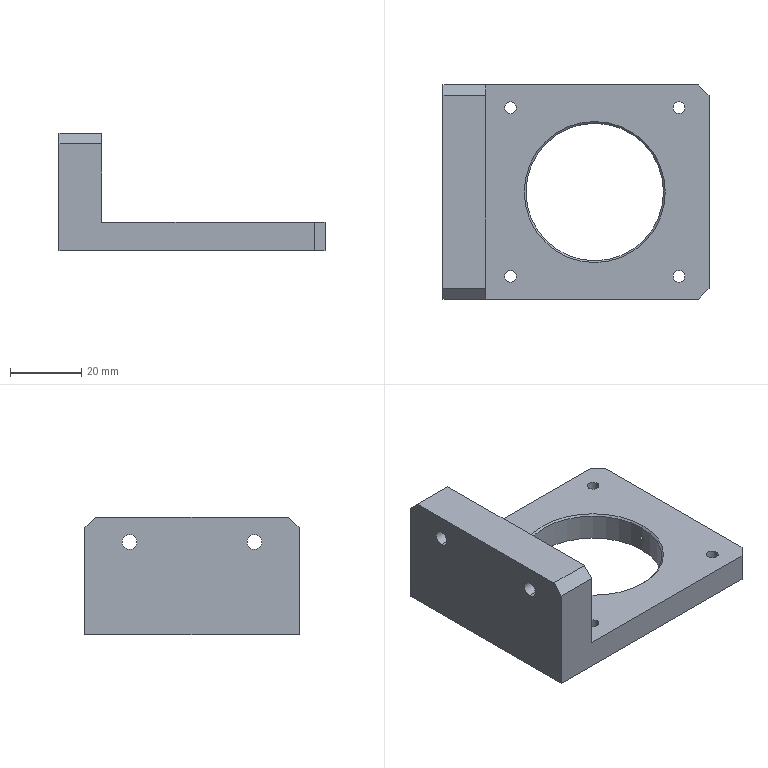Part | NX | features BREP 1 | 1 solid | 32 faces | box 74.5 x 60 x 33 mm | volume 43539 mm3 | cylinder 16 | plane 12 | cone 4 | commonest cylinder face diameters 3.3 x10 4.2 x4 38.5 x2
STEP:
#1=CARTESIAN_POINT('',(-42.5,-30.,30.));
#2=VERTEX_POINT('',#1);
#3=CARTESIAN_POINT('',(-42.5,-27.,33.));
#4=VERTEX_POINT('',#3);
#5=CARTESIAN_POINT('',(-42.5,-27.,33.));
#6=DIRECTION('',(0.,0.7071,0.7071));
#7=VECTOR('',#6,1000.);
#8=LINE('',#5,#7);
#9=EDGE_CURVE('',#2,#4,#8,.T.);
#10=ORIENTED_EDGE('',*,*,#9,.F.);
#11=CARTESIAN_POINT('',(-30.5,-30.,30.));
#12=VERTEX_POINT('',#11);
#13=CARTESIAN_POINT('',(-42.5,-30.,30.));
#14=DIRECTION('',(-1.,0.,0.));
#15=VECTOR('',#14,1000.);
#16=LINE('',#13,#15);
#17=EDGE_CURVE('',#12,#2,#16,.T.);
#18=ORIENTED_EDGE('',*,*,#17,.F.);
#19=CARTESIAN_POINT('',(-30.5,-27.,33.));
#20=VERTEX_POINT('',#19);
#21=CARTESIAN_POINT('',(-30.5,-27.,33.));
#22=DIRECTION('',(0.,-0.7071,-0.7071));
#23=VECTOR('',#22,1000.);
#24=LINE('',#21,#23);
#25=EDGE_CURVE('',#20,#12,#24,.T.);
#26=ORIENTED_EDGE('',*,*,#25,.F.);
#27=CARTESIAN_POINT('',(-30.5,-27.,33.));
#28=DIRECTION('',(1.,0.,0.));
#29=VECTOR('',#28,1000.);
#30=LINE('',#27,#29);
#31=EDGE_CURVE('',#4,#20,#30,.T.);
#32=ORIENTED_EDGE('',*,*,#31,.F.);
#33=EDGE_LOOP('',(#10,#18,#26,#32));
#34=FACE_BOUND('',#33,.T.);
#35=CARTESIAN_POINT('',(0.,-27.,33.));
#36=DIRECTION('',(0.,-0.7071,0.7071));
#37=DIRECTION('',(-1.,0.,0.));
#38=AXIS2_PLACEMENT_3D('',#35,#36,#37);
#39=PLANE('',#38);
#40=ADVANCED_FACE('',(#34),#39,.T.);
#41=CARTESIAN_POINT('',(-30.5,30.,30.));
#42=VERTEX_POINT('',#41);
#43=CARTESIAN_POINT('',(-30.5,27.,33.));
#44=VERTEX_POINT('',#43);
#45=CARTESIAN_POINT('',(-30.5,27.,33.));
#46=DIRECTION('',(0.,-0.7071,0.7071));
#47=VECTOR('',#46,1000.);
#48=LINE('',#45,#47);
#49=EDGE_CURVE('',#42,#44,#48,.T.);
#50=ORIENTED_EDGE('',*,*,#49,.F.);
#51=CARTESIAN_POINT('',(-42.5,30.,30.));
#52=VERTEX_POINT('',#51);
#53=CARTESIAN_POINT('',(-30.5,30.,30.));
#54=DIRECTION('',(1.,0.,0.));
#55=VECTOR('',#54,1000.);
#56=LINE('',#53,#55);
#57=EDGE_CURVE('',#52,#42,#56,.T.);
#58=ORIENTED_EDGE('',*,*,#57,.F.);
#59=CARTESIAN_POINT('',(-42.5,27.,33.));
#60=VERTEX_POINT('',#59);
#61=CARTESIAN_POINT('',(-42.5,27.,33.));
#62=DIRECTION('',(0.,0.7071,-0.7071));
#63=VECTOR('',#62,1000.);
#64=LINE('',#61,#63);
#65=EDGE_CURVE('',#60,#52,#64,.T.);
#66=ORIENTED_EDGE('',*,*,#65,.F.);
#67=CARTESIAN_POINT('',(-42.5,27.,33.));
#68=DIRECTION('',(-1.,0.,0.));
#69=VECTOR('',#68,1000.);
#70=LINE('',#67,#69);
#71=EDGE_CURVE('',#44,#60,#70,.T.);
#72=ORIENTED_EDGE('',*,*,#71,.F.);
#73=EDGE_LOOP('',(#50,#58,#66,#72));
#74=FACE_BOUND('',#73,.T.);
#75=CARTESIAN_POINT('',(0.,27.,33.));
#76=DIRECTION('',(0.,0.7071,0.7071));
#77=DIRECTION('',(1.,0.,0.));
#78=AXIS2_PLACEMENT_3D('',#75,#76,#77);
#79=PLANE('',#78);
#80=ADVANCED_FACE('',(#74),#79,.T.);
#81=CARTESIAN_POINT('',(29.,-30.,8.));
#82=VERTEX_POINT('',#81);
#83=CARTESIAN_POINT('',(32.,-27.,8.));
#84=VERTEX_POINT('',#83);
#85=CARTESIAN_POINT('',(32.,-27.,8.));
#86=DIRECTION('',(0.7071,0.7071,0.));
#87=VECTOR('',#86,1000.);
#88=LINE('',#85,#87);
#89=EDGE_CURVE('',#82,#84,#88,.T.);
#90=ORIENTED_EDGE('',*,*,#89,.F.);
#91=CARTESIAN_POINT('',(29.,-30.,0.));
#92=VERTEX_POINT('',#91);
#93=CARTESIAN_POINT('',(29.,-30.,8.));
#94=DIRECTION('',(0.,0.,1.));
#95=VECTOR('',#94,1000.);
#96=LINE('',#93,#95);
#97=EDGE_CURVE('',#92,#82,#96,.T.);
#98=ORIENTED_EDGE('',*,*,#97,.F.);
#99=CARTESIAN_POINT('',(32.,-27.,0.));
#100=VERTEX_POINT('',#99);
#101=CARTESIAN_POINT('',(29.5,-29.5,0.));
#102=DIRECTION('',(-0.7071,-0.7071,0.));
#103=VECTOR('',#102,1000.);
#104=LINE('',#101,#103);
#105=EDGE_CURVE('',#100,#92,#104,.T.);
#106=ORIENTED_EDGE('',*,*,#105,.F.);
#107=CARTESIAN_POINT('',(32.,-27.,8.));
#108=DIRECTION('',(0.,0.,-1.));
#109=VECTOR('',#108,1000.);
#110=LINE('',#107,#109);
#111=EDGE_CURVE('',#84,#100,#110,.T.);
#112=ORIENTED_EDGE('',*,*,#111,.F.);
#113=EDGE_LOOP('',(#90,#98,#106,#112));
#114=FACE_BOUND('',#113,.T.);
#115=CARTESIAN_POINT('',(32.,-27.,8.));
#116=DIRECTION('',(-0.7071,0.7071,0.));
#117=DIRECTION('',(0.,0.,-1.));
#118=AXIS2_PLACEMENT_3D('',#115,#116,#117);
#119=PLANE('',#118);
#120=ADVANCED_FACE('',(#114),#119,.F.);
#121=CARTESIAN_POINT('',(32.,27.,8.));
#122=VERTEX_POINT('',#121);
#123=CARTESIAN_POINT('',(29.,30.,8.));
#124=VERTEX_POINT('',#123);
#125=CARTESIAN_POINT('',(29.,30.,8.));
#126=DIRECTION('',(-0.7071,0.7071,0.));
#127=VECTOR('',#126,1000.);
#128=LINE('',#125,#127);
#129=EDGE_CURVE('',#122,#124,#128,.T.);
#130=ORIENTED_EDGE('',*,*,#129,.F.);
#131=CARTESIAN_POINT('',(32.,27.,0.));
#132=VERTEX_POINT('',#131);
#133=CARTESIAN_POINT('',(32.,27.,8.));
#134=DIRECTION('',(0.,0.,1.));
#135=VECTOR('',#134,1000.);
#136=LINE('',#133,#135);
#137=EDGE_CURVE('',#132,#122,#136,.T.);
#138=ORIENTED_EDGE('',*,*,#137,.F.);
#139=CARTESIAN_POINT('',(29.,30.,0.));
#140=VERTEX_POINT('',#139);
#141=CARTESIAN_POINT('',(29.5,29.5,0.));
#142=DIRECTION('',(0.7071,-0.7071,0.));
#143=VECTOR('',#142,1000.);
#144=LINE('',#141,#143);
#145=EDGE_CURVE('',#140,#132,#144,.T.);
#146=ORIENTED_EDGE('',*,*,#145,.F.);
#147=CARTESIAN_POINT('',(29.,30.,8.));
#148=DIRECTION('',(0.,0.,-1.));
#149=VECTOR('',#148,1000.);
#150=LINE('',#147,#149);
#151=EDGE_CURVE('',#124,#140,#150,.T.);
#152=ORIENTED_EDGE('',*,*,#151,.F.);
#153=EDGE_LOOP('',(#130,#138,#146,#152));
#154=FACE_BOUND('',#153,.T.);
#155=CARTESIAN_POINT('',(29.,30.,8.));
#156=DIRECTION('',(-0.7071,-0.7071,0.));
#157=DIRECTION('',(0.,0.,-1.));
#158=AXIS2_PLACEMENT_3D('',#155,#156,#157);
#159=PLANE('',#158);
#160=ADVANCED_FACE('',(#154),#159,.F.);
#161=CARTESIAN_POINT('',(19.9,0.,5.65));
#162=VERTEX_POINT('',#161);
#163=CARTESIAN_POINT('',(32.,0.,5.65));
#164=VERTEX_POINT('',#163);
#165=CARTESIAN_POINT('',(32.,0.,5.65));
#166=DIRECTION('',(1.,0.,0.));
#167=VECTOR('',#166,1000.);
#168=LINE('',#165,#167);
#169=EDGE_CURVE('',#162,#164,#168,.T.);
#170=ORIENTED_EDGE('',*,*,#169,.F.);
#171=CARTESIAN_POINT('',(19.9,0.,2.35));
#172=VERTEX_POINT('',#171);
#173=CARTESIAN_POINT('',(19.9,0.,4.));
#174=DIRECTION('',(1.,0.,0.));
#175=DIRECTION('',(0.,0.,-1.));
#176=AXIS2_PLACEMENT_3D('',#173,#174,#175);
#177=CIRCLE('',#176,1.65);
#178=EDGE_CURVE('',#172,#162,#177,.T.);
#179=ORIENTED_EDGE('',*,*,#178,.F.);
#180=CARTESIAN_POINT('',(32.,0.,2.35));
#181=VERTEX_POINT('',#180);
#182=CARTESIAN_POINT('',(32.,0.,2.35));
#183=DIRECTION('',(1.,0.,0.));
#184=VECTOR('',#183,1000.);
#185=LINE('',#182,#184);
#186=EDGE_CURVE('',#172,#181,#185,.T.);
#187=ORIENTED_EDGE('',*,*,#186,.T.);
#188=CARTESIAN_POINT('',(32.,0.,4.));
#189=DIRECTION('',(1.,0.,0.));
#190=DIRECTION('',(0.,0.,-1.));
#191=AXIS2_PLACEMENT_3D('',#188,#189,#190);
#192=CIRCLE('',#191,1.65);
#193=EDGE_CURVE('',#181,#164,#192,.T.);
#194=ORIENTED_EDGE('',*,*,#193,.T.);
#195=EDGE_LOOP('',(#170,#179,#187,#194));
#196=FACE_BOUND('',#195,.T.);
#197=CARTESIAN_POINT('',(32.,0.,4.));
#198=DIRECTION('',(1.,0.,0.));
#199=DIRECTION('',(0.,0.,-1.));
#200=AXIS2_PLACEMENT_3D('',#197,#198,#199);
#201=CYLINDRICAL_SURFACE('',#200,1.65);
#202=ADVANCED_FACE('',(#196),#201,.F.);
#203=CARTESIAN_POINT('',(19.25,0.,4.568));
#204=VERTEX_POINT('',#203);
#205=CARTESIAN_POINT('',(19.9,0.,5.65));
#206=DIRECTION('',(0.515,0.,0.8572));
#207=VECTOR('',#206,1000.);
#208=LINE('',#205,#207);
#209=EDGE_CURVE('',#204,#162,#208,.T.);
#210=ORIENTED_EDGE('',*,*,#209,.F.);
#211=CARTESIAN_POINT('',(19.25,0.,3.432));
#212=VERTEX_POINT('',#211);
#213=CARTESIAN_POINT('',(19.25,0.,3.432));
#214=CARTESIAN_POINT('',(19.25,0.2923,3.432));
#215=CARTESIAN_POINT('',(19.234,0.8169,4.));
#216=CARTESIAN_POINT('',(19.25,0.2935,4.568));
#217=CARTESIAN_POINT('',(19.25,0.,4.568));
#218=B_SPLINE_CURVE_WITH_KNOTS('',3,(#213,#214,#215,#216,#217),.UNSPECIFIED.,.F.,.F.,(4,1,4),(0.,0.5,1.),.UNSPECIFIED.);
#219=EDGE_CURVE('',#204,#212,#218,.F.);
#220=ORIENTED_EDGE('',*,*,#219,.T.);
#221=CARTESIAN_POINT('',(19.9,0.,2.35));
#222=DIRECTION('',(0.515,0.,-0.8572));
#223=VECTOR('',#222,1000.);
#224=LINE('',#221,#223);
#225=EDGE_CURVE('',#212,#172,#224,.T.);
#226=ORIENTED_EDGE('',*,*,#225,.T.);
#227=ORIENTED_EDGE('',*,*,#178,.T.);
#228=EDGE_LOOP('',(#210,#220,#226,#227));
#229=FACE_BOUND('',#228,.T.);
#230=CARTESIAN_POINT('',(19.9,0.,4.));
#231=DIRECTION('',(1.,0.,0.));
#232=DIRECTION('',(0.,0.,-1.));
#233=AXIS2_PLACEMENT_3D('',#230,#231,#232);
#234=CONICAL_SURFACE('',#233,1.65,1.03);
#235=ADVANCED_FACE('',(#229),#234,.F.);
#236=CARTESIAN_POINT('',(-42.5,17.5,23.9));
#237=VERTEX_POINT('',#236);
#238=CARTESIAN_POINT('',(-30.5,17.5,23.9));
#239=VERTEX_POINT('',#238);
#240=CARTESIAN_POINT('',(-42.5,17.5,23.9));
#241=DIRECTION('',(-1.,0.,0.));
#242=VECTOR('',#241,1000.);
#243=LINE('',#240,#242);
#244=EDGE_CURVE('',#237,#239,#243,.F.);
#245=ORIENTED_EDGE('',*,*,#244,.T.);
#246=CARTESIAN_POINT('',(-30.5,17.5,28.1));
#247=VERTEX_POINT('',#246);
#248=CARTESIAN_POINT('',(-30.5,17.5,26.));
#249=DIRECTION('',(-1.,0.,0.));
#250=DIRECTION('',(0.,-1.,0.));
#251=AXIS2_PLACEMENT_3D('',#248,#249,#250);
#252=CIRCLE('',#251,2.1);
#253=EDGE_CURVE('',#247,#239,#252,.T.);
#254=ORIENTED_EDGE('',*,*,#253,.F.);
#255=CARTESIAN_POINT('',(-42.5,17.5,28.1));
#256=VERTEX_POINT('',#255);
#257=CARTESIAN_POINT('',(-42.5,17.5,28.1));
#258=DIRECTION('',(-1.,0.,0.));
#259=VECTOR('',#258,1000.);
#260=LINE('',#257,#259);
#261=EDGE_CURVE('',#256,#247,#260,.F.);
#262=ORIENTED_EDGE('',*,*,#261,.F.);
#263=CARTESIAN_POINT('',(-42.5,17.5,26.));
#264=DIRECTION('',(-1.,0.,0.));
#265=DIRECTION('',(0.,0.,1.));
#266=AXIS2_PLACEMENT_3D('',#263,#264,#265);
#267=CIRCLE('',#266,2.1);
#268=EDGE_CURVE('',#256,#237,#267,.T.);
#269=ORIENTED_EDGE('',*,*,#268,.T.);
#270=EDGE_LOOP('',(#245,#254,#262,#269));
#271=FACE_BOUND('',#270,.T.);
#272=CARTESIAN_POINT('',(-42.5,17.5,26.));
#273=DIRECTION('',(-1.,0.,0.));
#274=DIRECTION('',(0.,0.,1.));
#275=AXIS2_PLACEMENT_3D('',#272,#273,#274);
#276=CYLINDRICAL_SURFACE('',#275,2.1);
#277=ADVANCED_FACE('',(#271),#276,.F.);
#278=CARTESIAN_POINT('',(-42.5,-17.5,23.9));
#279=VERTEX_POINT('',#278);
#280=CARTESIAN_POINT('',(-30.5,-17.5,23.9));
#281=VERTEX_POINT('',#280);
#282=CARTESIAN_POINT('',(-42.5,-17.5,23.9));
#283=DIRECTION('',(-1.,0.,0.));
#284=VECTOR('',#283,1000.);
#285=LINE('',#282,#284);
#286=EDGE_CURVE('',#279,#281,#285,.F.);
#287=ORIENTED_EDGE('',*,*,#286,.T.);
#288=CARTESIAN_POINT('',(-30.5,-17.5,28.1));
#289=VERTEX_POINT('',#288);
#290=CARTESIAN_POINT('',(-30.5,-17.5,26.));
#291=DIRECTION('',(-1.,0.,0.));
#292=DIRECTION('',(0.,-1.,0.));
#293=AXIS2_PLACEMENT_3D('',#290,#291,#292);
#294=CIRCLE('',#293,2.1);
#295=EDGE_CURVE('',#289,#281,#294,.T.);
#296=ORIENTED_EDGE('',*,*,#295,.F.);
#297=CARTESIAN_POINT('',(-42.5,-17.5,28.1));
#298=VERTEX_POINT('',#297);
#299=CARTESIAN_POINT('',(-42.5,-17.5,28.1));
#300=DIRECTION('',(-1.,0.,0.));
#301=VECTOR('',#300,1000.);
#302=LINE('',#299,#301);
#303=EDGE_CURVE('',#298,#289,#302,.F.);
#304=ORIENTED_EDGE('',*,*,#303,.F.);
#305=CARTESIAN_POINT('',(-42.5,-17.5,26.));
#306=DIRECTION('',(-1.,0.,0.));
#307=DIRECTION('',(0.,0.,1.));
#308=AXIS2_PLACEMENT_3D('',#305,#306,#307);
#309=CIRCLE('',#308,2.1);
#310=EDGE_CURVE('',#298,#279,#309,.T.);
#311=ORIENTED_EDGE('',*,*,#310,.T.);
#312=EDGE_LOOP('',(#287,#296,#304,#311));
#313=FACE_BOUND('',#312,.T.);
#314=CARTESIAN_POINT('',(-42.5,-17.5,26.));
#315=DIRECTION('',(-1.,0.,0.));
#316=DIRECTION('',(0.,0.,1.));
#317=AXIS2_PLACEMENT_3D('',#314,#315,#316);
#318=CYLINDRICAL_SURFACE('',#317,2.1);
#319=ADVANCED_FACE('',(#313),#318,.F.);
#320=CARTESIAN_POINT('',(-19.75,0.,8.));
#321=VERTEX_POINT('',#320);
#322=CARTESIAN_POINT('',(-19.25,0.,7.5));
#323=VERTEX_POINT('',#322);
#324=CARTESIAN_POINT('',(-19.25,0.,7.5));
#325=DIRECTION('',(-0.7071,0.,0.7071));
#326=VECTOR('',#325,1000.);
#327=LINE('',#324,#326);
#328=EDGE_CURVE('',#321,#323,#327,.F.);
#329=ORIENTED_EDGE('',*,*,#328,.T.);
#330=CARTESIAN_POINT('',(19.25,0.,7.5));
#331=VERTEX_POINT('',#330);
#332=CARTESIAN_POINT('',(0.,0.,7.5));
#333=DIRECTION('',(0.,0.,1.));
#334=DIRECTION('',(-1.,0.,0.));
#335=AXIS2_PLACEMENT_3D('',#332,#333,#334);
#336=CIRCLE('',#335,19.25);
#337=EDGE_CURVE('',#331,#323,#336,.T.);
#338=ORIENTED_EDGE('',*,*,#337,.F.);
#339=CARTESIAN_POINT('',(19.75,0.,8.));
#340=VERTEX_POINT('',#339);
#341=CARTESIAN_POINT('',(19.25,0.,7.5));
#342=DIRECTION('',(0.7071,0.,0.7071));
#343=VECTOR('',#342,1000.);
#344=LINE('',#341,#343);
#345=EDGE_CURVE('',#340,#331,#344,.F.);
#346=ORIENTED_EDGE('',*,*,#345,.F.);
#347=CARTESIAN_POINT('',(0.,0.,8.));
#348=DIRECTION('',(0.,0.,-1.));
#349=DIRECTION('',(-1.,0.,0.));
#350=AXIS2_PLACEMENT_3D('',#347,#348,#349);
#351=CIRCLE('',#350,19.75);
#352=EDGE_CURVE('',#321,#340,#351,.T.);
#353=ORIENTED_EDGE('',*,*,#352,.F.);
#354=EDGE_LOOP('',(#329,#338,#346,#353));
#355=FACE_BOUND('',#354,.T.);
#356=CARTESIAN_POINT('',(0.,0.,7.5));
#357=DIRECTION('',(0.,0.,1.));
#358=DIRECTION('',(1.,0.,0.));
#359=AXIS2_PLACEMENT_3D('',#356,#357,#358);
#360=CONICAL_SURFACE('',#359,19.25,0.7854);
#361=ADVANCED_FACE('',(#355),#360,.F.);
#362=CARTESIAN_POINT('',(-21.95,23.6,8.));
#363=VERTEX_POINT('',#362);
#364=CARTESIAN_POINT('',(-21.95,23.6,0.));
#365=VERTEX_POINT('',#364);
#366=CARTESIAN_POINT('',(-21.95,23.6,0.));
#367=DIRECTION('',(0.,0.,-1.));
#368=VECTOR('',#367,1000.);
#369=LINE('',#366,#368);
#370=EDGE_CURVE('',#363,#365,#369,.T.);
#371=ORIENTED_EDGE('',*,*,#370,.F.);
#372=CARTESIAN_POINT('',(-25.25,23.6,8.));
#373=VERTEX_POINT('',#372);
#374=CARTESIAN_POINT('',(-23.6,23.6,8.));
#375=DIRECTION('',(0.,0.,-1.));
#376=DIRECTION('',(-1.,0.,0.));
#377=AXIS2_PLACEMENT_3D('',#374,#375,#376);
#378=CIRCLE('',#377,1.65);
#379=EDGE_CURVE('',#373,#363,#378,.T.);
#380=ORIENTED_EDGE('',*,*,#379,.F.);
#381=CARTESIAN_POINT('',(-25.25,23.6,0.));
#382=VERTEX_POINT('',#381);
#383=CARTESIAN_POINT('',(-25.25,23.6,0.));
#384=DIRECTION('',(0.,0.,-1.));
#385=VECTOR('',#384,1000.);
#386=LINE('',#383,#385);
#387=EDGE_CURVE('',#373,#382,#386,.T.);
#388=ORIENTED_EDGE('',*,*,#387,.T.);
#389=CARTESIAN_POINT('',(-23.6,23.6,0.));
#390=DIRECTION('',(0.,0.,-1.));
#391=DIRECTION('',(-1.,0.,0.));
#392=AXIS2_PLACEMENT_3D('',#389,#390,#391);
#393=CIRCLE('',#392,1.65);
#394=EDGE_CURVE('',#382,#365,#393,.T.);
#395=ORIENTED_EDGE('',*,*,#394,.T.);
#396=EDGE_LOOP('',(#371,#380,#388,#395));
#397=FACE_BOUND('',#396,.T.);
#398=CARTESIAN_POINT('',(-23.6,23.6,0.));
#399=DIRECTION('',(0.,0.,-1.));
#400=DIRECTION('',(-1.,0.,0.));
#401=AXIS2_PLACEMENT_3D('',#398,#399,#400);
#402=CYLINDRICAL_SURFACE('',#401,1.65);
#403=ADVANCED_FACE('',(#397),#402,.F.);
#404=CARTESIAN_POINT('',(25.25,-23.6,8.));
#405=VERTEX_POINT('',#404);
#406=CARTESIAN_POINT('',(25.25,-23.6,0.));
#407=VERTEX_POINT('',#406);
#408=CARTESIAN_POINT('',(25.25,-23.6,0.));
#409=DIRECTION('',(0.,0.,-1.));
#410=VECTOR('',#409,1000.);
#411=LINE('',#408,#410);
#412=EDGE_CURVE('',#405,#407,#411,.T.);
#413=ORIENTED_EDGE('',*,*,#412,.F.);
#414=CARTESIAN_POINT('',(21.95,-23.6,8.));
#415=VERTEX_POINT('',#414);
#416=CARTESIAN_POINT('',(23.6,-23.6,8.));
#417=DIRECTION('',(0.,0.,-1.));
#418=DIRECTION('',(-1.,0.,0.));
#419=AXIS2_PLACEMENT_3D('',#416,#417,#418);
#420=CIRCLE('',#419,1.65);
#421=EDGE_CURVE('',#415,#405,#420,.T.);
#422=ORIENTED_EDGE('',*,*,#421,.F.);
#423=CARTESIAN_POINT('',(21.95,-23.6,0.));
#424=VERTEX_POINT('',#423);
#425=CARTESIAN_POINT('',(21.95,-23.6,0.));
#426=DIRECTION('',(0.,0.,-1.));
#427=VECTOR('',#426,1000.);
#428=LINE('',#425,#427);
#429=EDGE_CURVE('',#415,#424,#428,.T.);
#430=ORIENTED_EDGE('',*,*,#429,.T.);
#431=CARTESIAN_POINT('',(23.6,-23.6,0.));
#432=DIRECTION('',(0.,0.,-1.));
#433=DIRECTION('',(-1.,0.,0.));
#434=AXIS2_PLACEMENT_3D('',#431,#432,#433);
#435=CIRCLE('',#434,1.65);
#436=EDGE_CURVE('',#424,#407,#435,.T.);
#437=ORIENTED_EDGE('',*,*,#436,.T.);
#438=EDGE_LOOP('',(#413,#422,#430,#437));
#439=FACE_BOUND('',#438,.T.);
#440=CARTESIAN_POINT('',(23.6,-23.6,0.));
#441=DIRECTION('',(0.,0.,-1.));
#442=DIRECTION('',(-1.,0.,0.));
#443=AXIS2_PLACEMENT_3D('',#440,#441,#442);
#444=CYLINDRICAL_SURFACE('',#443,1.65);
#445=ADVANCED_FACE('',(#439),#444,.F.);
#446=CARTESIAN_POINT('',(25.25,23.6,8.));
#447=VERTEX_POINT('',#446);
#448=CARTESIAN_POINT('',(25.25,23.6,0.));
#449=VERTEX_POINT('',#448);
#450=CARTESIAN_POINT('',(25.25,23.6,0.));
#451=DIRECTION('',(0.,0.,-1.));
#452=VECTOR('',#451,1000.);
#453=LINE('',#450,#452);
#454=EDGE_CURVE('',#447,#449,#453,.T.);
#455=ORIENTED_EDGE('',*,*,#454,.F.);
#456=CARTESIAN_POINT('',(21.95,23.6,8.));
#457=VERTEX_POINT('',#456);
#458=CARTESIAN_POINT('',(23.6,23.6,8.));
#459=DIRECTION('',(0.,0.,-1.));
#460=DIRECTION('',(-1.,0.,0.));
#461=AXIS2_PLACEMENT_3D('',#458,#459,#460);
#462=CIRCLE('',#461,1.65);
#463=EDGE_CURVE('',#457,#447,#462,.T.);
#464=ORIENTED_EDGE('',*,*,#463,.F.);
#465=CARTESIAN_POINT('',(21.95,23.6,0.));
#466=VERTEX_POINT('',#465);
#467=CARTESIAN_POINT('',(21.95,23.6,0.));
#468=DIRECTION('',(0.,0.,-1.));
#469=VECTOR('',#468,1000.);
#470=LINE('',#467,#469);
#471=EDGE_CURVE('',#457,#466,#470,.T.);
#472=ORIENTED_EDGE('',*,*,#471,.T.);
#473=CARTESIAN_POINT('',(23.6,23.6,0.));
#474=DIRECTION('',(0.,0.,-1.));
#475=DIRECTION('',(-1.,0.,0.));
#476=AXIS2_PLACEMENT_3D('',#473,#474,#475);
#477=CIRCLE('',#476,1.65);
#478=EDGE_CURVE('',#466,#449,#477,.T.);
#479=ORIENTED_EDGE('',*,*,#478,.T.);
#480=EDGE_LOOP('',(#455,#464,#472,#479));
#481=FACE_BOUND('',#480,.T.);
#482=CARTESIAN_POINT('',(23.6,23.6,0.));
#483=DIRECTION('',(0.,0.,-1.));
#484=DIRECTION('',(-1.,0.,0.));
#485=AXIS2_PLACEMENT_3D('',#482,#483,#484);
#486=CYLINDRICAL_SURFACE('',#485,1.65);
#487=ADVANCED_FACE('',(#481),#486,.F.);
#488=CARTESIAN_POINT('',(-21.95,-23.6,8.));
#489=VERTEX_POINT('',#488);
#490=CARTESIAN_POINT('',(-21.95,-23.6,0.));
#491=VERTEX_POINT('',#490);
#492=CARTESIAN_POINT('',(-21.95,-23.6,0.));
#493=DIRECTION('',(0.,0.,-1.));
#494=VECTOR('',#493,1000.);
#495=LINE('',#492,#494);
#496=EDGE_CURVE('',#489,#491,#495,.T.);
#497=ORIENTED_EDGE('',*,*,#496,.F.);
#498=CARTESIAN_POINT('',(-25.25,-23.6,8.));
#499=VERTEX_POINT('',#498);
#500=CARTESIAN_POINT('',(-23.6,-23.6,8.));
#501=DIRECTION('',(0.,0.,-1.));
#502=DIRECTION('',(-1.,0.,0.));
#503=AXIS2_PLACEMENT_3D('',#500,#501,#502);
#504=CIRCLE('',#503,1.65);
#505=EDGE_CURVE('',#499,#489,#504,.T.);
#506=ORIENTED_EDGE('',*,*,#505,.F.);
#507=CARTESIAN_POINT('',(-25.25,-23.6,0.));
#508=VERTEX_POINT('',#507);
#509=CARTESIAN_POINT('',(-25.25,-23.6,0.));
#510=DIRECTION('',(0.,0.,-1.));
#511=VECTOR('',#510,1000.);
#512=LINE('',#509,#511);
#513=EDGE_CURVE('',#499,#508,#512,.T.);
#514=ORIENTED_EDGE('',*,*,#513,.T.);
#515=CARTESIAN_POINT('',(-23.6,-23.6,0.));
#516=DIRECTION('',(0.,0.,-1.));
#517=DIRECTION('',(-1.,0.,0.));
#518=AXIS2_PLACEMENT_3D('',#515,#516,#517);
#519=CIRCLE('',#518,1.65);
#520=EDGE_CURVE('',#508,#491,#519,.T.);
#521=ORIENTED_EDGE('',*,*,#520,.T.);
#522=EDGE_LOOP('',(#497,#506,#514,#521));
#523=FACE_BOUND('',#522,.T.);
#524=CARTESIAN_POINT('',(-23.6,-23.6,0.));
#525=DIRECTION('',(0.,0.,-1.));
#526=DIRECTION('',(-1.,0.,0.));
#527=AXIS2_PLACEMENT_3D('',#524,#525,#526);
#528=CYLINDRICAL_SURFACE('',#527,1.65);
#529=ADVANCED_FACE('',(#523),#528,.F.);
#530=CARTESIAN_POINT('',(-30.5,30.,33.));
#531=DIRECTION('',(0.,1.,0.));
#532=VECTOR('',#531,1000.);
#533=LINE('',#530,#532);
#534=EDGE_CURVE('',#20,#44,#533,.T.);
#535=ORIENTED_EDGE('',*,*,#534,.T.);
#536=ORIENTED_EDGE('',*,*,#71,.T.);
#537=CARTESIAN_POINT('',(-42.5,30.,33.));
#538=DIRECTION('',(0.,-1.,0.));
#539=VECTOR('',#538,1000.);
#540=LINE('',#537,#539);
#541=EDGE_CURVE('',#60,#4,#540,.T.);
#542=ORIENTED_EDGE('',*,*,#541,.T.);
#543=ORIENTED_EDGE('',*,*,#31,.T.);
#544=EDGE_LOOP('',(#535,#536,#542,#543));
#545=FACE_BOUND('',#544,.T.);
#546=CARTESIAN_POINT('',(0.,0.,33.));
#547=DIRECTION('',(0.,0.,1.));
#548=DIRECTION('',(1.,0.,0.));
#549=AXIS2_PLACEMENT_3D('',#546,#547,#548);
#550=PLANE('',#549);
#551=ADVANCED_FACE('',(#545),#550,.T.);
#552=CARTESIAN_POINT('',(-30.5,30.,8.));
#553=VERTEX_POINT('',#552);
#554=CARTESIAN_POINT('',(-30.5,30.,33.));
#555=DIRECTION('',(0.,0.,-1.));
#556=VECTOR('',#555,1000.);
#557=LINE('',#554,#556);
#558=EDGE_CURVE('',#42,#553,#557,.T.);
#559=ORIENTED_EDGE('',*,*,#558,.F.);
#560=ORIENTED_EDGE('',*,*,#49,.T.);
#561=ORIENTED_EDGE('',*,*,#534,.F.);
#562=ORIENTED_EDGE('',*,*,#25,.T.);
#563=CARTESIAN_POINT('',(-30.5,-30.,8.));
#564=VERTEX_POINT('',#563);
#565=CARTESIAN_POINT('',(-30.5,-30.,33.));
#566=DIRECTION('',(0.,0.,-1.));
#567=VECTOR('',#566,1000.);
#568=LINE('',#565,#567);
#569=EDGE_CURVE('',#12,#564,#568,.T.);
#570=ORIENTED_EDGE('',*,*,#569,.T.);
#571=CARTESIAN_POINT('',(-30.5,30.,8.));
#572=DIRECTION('',(0.,1.,0.));
#573=VECTOR('',#572,1000.);
#574=LINE('',#571,#573);
#575=EDGE_CURVE('',#564,#553,#574,.T.);
#576=ORIENTED_EDGE('',*,*,#575,.T.);
#577=EDGE_LOOP('',(#559,#560,#561,#562,#570,#576));
#578=FACE_BOUND('',#577,.T.);
#579=ORIENTED_EDGE('',*,*,#295,.T.);
#580=CARTESIAN_POINT('',(-30.5,-17.5,26.));
#581=DIRECTION('',(-1.,0.,0.));
#582=DIRECTION('',(0.,-1.,0.));
#583=AXIS2_PLACEMENT_3D('',#580,#581,#582);
#584=CIRCLE('',#583,2.1);
#585=EDGE_CURVE('',#281,#289,#584,.T.);
#586=ORIENTED_EDGE('',*,*,#585,.T.);
#587=EDGE_LOOP('',(#579,#586));
#588=FACE_BOUND('',#587,.T.);
#589=ORIENTED_EDGE('',*,*,#253,.T.);
#590=CARTESIAN_POINT('',(-30.5,17.5,26.));
#591=DIRECTION('',(-1.,0.,0.));
#592=DIRECTION('',(0.,-1.,0.));
#593=AXIS2_PLACEMENT_3D('',#590,#591,#592);
#594=CIRCLE('',#593,2.1);
#595=EDGE_CURVE('',#239,#247,#594,.T.);
#596=ORIENTED_EDGE('',*,*,#595,.T.);
#597=EDGE_LOOP('',(#589,#596));
#598=FACE_BOUND('',#597,.T.);
#599=CARTESIAN_POINT('',(-30.5,30.,33.));
#600=DIRECTION('',(-1.,0.,0.));
#601=DIRECTION('',(0.,-1.,0.));
#602=AXIS2_PLACEMENT_3D('',#599,#600,#601);
#603=PLANE('',#602);
#604=ADVANCED_FACE('',(#578,#588,#598),#603,.F.);
#605=CARTESIAN_POINT('',(19.25,0.,8.));
#606=DIRECTION('',(0.,0.,-1.));
#607=VECTOR('',#606,1000.);
#608=LINE('',#605,#607);
#609=EDGE_CURVE('',#331,#204,#608,.T.);
#610=ORIENTED_EDGE('',*,*,#609,.F.);
#611=ORIENTED_EDGE('',*,*,#337,.T.);
#612=CARTESIAN_POINT('',(-19.25,0.,0.));
#613=VERTEX_POINT('',#612);
#614=CARTESIAN_POINT('',(-19.25,0.,8.));
#615=DIRECTION('',(0.,0.,-1.));
#616=VECTOR('',#615,1000.);
#617=LINE('',#614,#616);
#618=EDGE_CURVE('',#323,#613,#617,.T.);
#619=ORIENTED_EDGE('',*,*,#618,.T.);
#620=CARTESIAN_POINT('',(19.25,0.,0.));
#621=VERTEX_POINT('',#620);
#622=CARTESIAN_POINT('',(0.,0.,0.));
#623=DIRECTION('',(0.,0.,1.));
#624=DIRECTION('',(1.,0.,0.));
#625=AXIS2_PLACEMENT_3D('',#622,#623,#624);
#626=CIRCLE('',#625,19.25);
#627=EDGE_CURVE('',#621,#613,#626,.T.);
#628=ORIENTED_EDGE('',*,*,#627,.F.);
#629=CARTESIAN_POINT('',(19.25,0.,8.));
#630=DIRECTION('',(0.,0.,-1.));
#631=VECTOR('',#630,1000.);
#632=LINE('',#629,#631);
#633=EDGE_CURVE('',#212,#621,#632,.T.);
#634=ORIENTED_EDGE('',*,*,#633,.F.);
#635=ORIENTED_EDGE('',*,*,#219,.F.);
#636=EDGE_LOOP('',(#610,#611,#619,#628,#634,#635));
#637=FACE_BOUND('',#636,.T.);
#638=CARTESIAN_POINT('',(0.,0.,8.));
#639=DIRECTION('',(0.,0.,-1.));
#640=DIRECTION('',(-1.,0.,0.));
#641=AXIS2_PLACEMENT_3D('',#638,#639,#640);
#642=CYLINDRICAL_SURFACE('',#641,19.25);
#643=ADVANCED_FACE('',(#637),#642,.F.);
#644=CARTESIAN_POINT('',(-42.5,-30.,0.));
#645=VERTEX_POINT('',#644);
#646=CARTESIAN_POINT('',(-42.5,-30.,0.));
#647=DIRECTION('',(1.,0.,0.));
#648=VECTOR('',#647,1000.);
#649=LINE('',#646,#648);
#650=EDGE_CURVE('',#645,#92,#649,.T.);
#651=ORIENTED_EDGE('',*,*,#650,.T.);
#652=ORIENTED_EDGE('',*,*,#97,.T.);
#653=CARTESIAN_POINT('',(-42.5,-30.,8.));
#654=DIRECTION('',(1.,0.,0.));
#655=VECTOR('',#654,1000.);
#656=LINE('',#653,#655);
#657=EDGE_CURVE('',#564,#82,#656,.T.);
#658=ORIENTED_EDGE('',*,*,#657,.F.);
#659=ORIENTED_EDGE('',*,*,#569,.F.);
#660=ORIENTED_EDGE('',*,*,#17,.T.);
#661=CARTESIAN_POINT('',(-42.5,-30.,8.));
#662=DIRECTION('',(0.,0.,-1.));
#663=VECTOR('',#662,1000.);
#664=LINE('',#661,#663);
#665=EDGE_CURVE('',#2,#645,#664,.T.);
#666=ORIENTED_EDGE('',*,*,#665,.T.);
#667=EDGE_LOOP('',(#651,#652,#658,#659,#660,#666));
#668=FACE_BOUND('',#667,.T.);
#669=CARTESIAN_POINT('',(-42.5,-30.,8.));
#670=DIRECTION('',(0.,1.,0.));
#671=DIRECTION('',(-1.,0.,0.));
#672=AXIS2_PLACEMENT_3D('',#669,#670,#671);
#673=PLANE('',#672);
#674=ADVANCED_FACE('',(#668),#673,.F.);
#675=CARTESIAN_POINT('',(-42.5,30.,8.));
#676=DIRECTION('',(-1.,0.,0.));
#677=VECTOR('',#676,1000.);
#678=LINE('',#675,#677);
#679=EDGE_CURVE('',#124,#553,#678,.T.);
#680=ORIENTED_EDGE('',*,*,#679,.F.);
#681=ORIENTED_EDGE('',*,*,#151,.T.);
#682=CARTESIAN_POINT('',(-42.5,30.,0.));
#683=VERTEX_POINT('',#682);
#684=CARTESIAN_POINT('',(-42.5,30.,0.));
#685=DIRECTION('',(-1.,0.,0.));
#686=VECTOR('',#685,1000.);
#687=LINE('',#684,#686);
#688=EDGE_CURVE('',#140,#683,#687,.T.);
#689=ORIENTED_EDGE('',*,*,#688,.T.);
#690=CARTESIAN_POINT('',(-42.5,30.,8.));
#691=DIRECTION('',(0.,0.,-1.));
#692=VECTOR('',#691,1000.);
#693=LINE('',#690,#692);
#694=EDGE_CURVE('',#52,#683,#693,.T.);
#695=ORIENTED_EDGE('',*,*,#694,.F.);
#696=ORIENTED_EDGE('',*,*,#57,.T.);
#697=ORIENTED_EDGE('',*,*,#558,.T.);
#698=EDGE_LOOP('',(#680,#681,#689,#695,#696,#697));
#699=FACE_BOUND('',#698,.T.);
#700=CARTESIAN_POINT('',(-42.5,30.,8.));
#701=DIRECTION('',(0.,-1.,0.));
#702=DIRECTION('',(1.,0.,0.));
#703=AXIS2_PLACEMENT_3D('',#700,#701,#702);
#704=PLANE('',#703);
#705=ADVANCED_FACE('',(#699),#704,.F.);
#706=CARTESIAN_POINT('',(32.,-30.,0.));
#707=DIRECTION('',(0.,1.,0.));
#708=VECTOR('',#707,1000.);
#709=LINE('',#706,#708);
#710=EDGE_CURVE('',#100,#132,#709,.T.);
#711=ORIENTED_EDGE('',*,*,#710,.T.);
#712=ORIENTED_EDGE('',*,*,#137,.T.);
#713=CARTESIAN_POINT('',(32.,-30.,8.));
#714=DIRECTION('',(0.,1.,0.));
#715=VECTOR('',#714,1000.);
#716=LINE('',#713,#715);
#717=EDGE_CURVE('',#84,#122,#716,.T.);
#718=ORIENTED_EDGE('',*,*,#717,.F.);
#719=ORIENTED_EDGE('',*,*,#111,.T.);
#720=EDGE_LOOP('',(#711,#712,#718,#719));
#721=FACE_BOUND('',#720,.T.);
#722=ORIENTED_EDGE('',*,*,#193,.F.);
#723=CARTESIAN_POINT('',(32.,0.,4.));
#724=DIRECTION('',(1.,0.,0.));
#725=DIRECTION('',(0.,0.,-1.));
#726=AXIS2_PLACEMENT_3D('',#723,#724,#725);
#727=CIRCLE('',#726,1.65);
#728=EDGE_CURVE('',#164,#181,#727,.T.);
#729=ORIENTED_EDGE('',*,*,#728,.F.);
#730=EDGE_LOOP('',(#722,#729));
#731=FACE_BOUND('',#730,.T.);
#732=CARTESIAN_POINT('',(32.,-30.,8.));
#733=DIRECTION('',(-1.,0.,0.));
#734=DIRECTION('',(0.,-1.,0.));
#735=AXIS2_PLACEMENT_3D('',#732,#733,#734);
#736=PLANE('',#735);
#737=ADVANCED_FACE('',(#721,#731),#736,.F.);
#738=CARTESIAN_POINT('',(0.,0.,0.));
#739=DIRECTION('',(0.,0.,1.));
#740=DIRECTION('',(1.,0.,0.));
#741=AXIS2_PLACEMENT_3D('',#738,#739,#740);
#742=CIRCLE('',#741,19.25);
#743=EDGE_CURVE('',#613,#621,#742,.T.);
#744=ORIENTED_EDGE('',*,*,#743,.T.);
#745=ORIENTED_EDGE('',*,*,#627,.T.);
#746=EDGE_LOOP('',(#744,#745));
#747=FACE_BOUND('',#746,.T.);
#748=ORIENTED_EDGE('',*,*,#688,.F.);
#749=ORIENTED_EDGE('',*,*,#145,.T.);
#750=ORIENTED_EDGE('',*,*,#710,.F.);
#751=ORIENTED_EDGE('',*,*,#105,.T.);
#752=ORIENTED_EDGE('',*,*,#650,.F.);
#753=CARTESIAN_POINT('',(-42.5,-30.,0.));
#754=DIRECTION('',(0.,-1.,0.));
#755=VECTOR('',#754,1000.);
#756=LINE('',#753,#755);
#757=EDGE_CURVE('',#683,#645,#756,.T.);
#758=ORIENTED_EDGE('',*,*,#757,.F.);
#759=EDGE_LOOP('',(#748,#749,#750,#751,#752,#758));
#760=FACE_BOUND('',#759,.T.);
#761=ORIENTED_EDGE('',*,*,#520,.F.);
#762=CARTESIAN_POINT('',(-23.6,-23.6,0.));
#763=DIRECTION('',(0.,0.,-1.));
#764=DIRECTION('',(-1.,0.,0.));
#765=AXIS2_PLACEMENT_3D('',#762,#763,#764);
#766=CIRCLE('',#765,1.65);
#767=EDGE_CURVE('',#491,#508,#766,.T.);
#768=ORIENTED_EDGE('',*,*,#767,.F.);
#769=EDGE_LOOP('',(#761,#768));
#770=FACE_BOUND('',#769,.T.);
#771=ORIENTED_EDGE('',*,*,#478,.F.);
#772=CARTESIAN_POINT('',(23.6,23.6,0.));
#773=DIRECTION('',(0.,0.,-1.));
#774=DIRECTION('',(-1.,0.,0.));
#775=AXIS2_PLACEMENT_3D('',#772,#773,#774);
#776=CIRCLE('',#775,1.65);
#777=EDGE_CURVE('',#449,#466,#776,.T.);
#778=ORIENTED_EDGE('',*,*,#777,.F.);
#779=EDGE_LOOP('',(#771,#778));
#780=FACE_BOUND('',#779,.T.);
#781=ORIENTED_EDGE('',*,*,#436,.F.);
#782=CARTESIAN_POINT('',(23.6,-23.6,0.));
#783=DIRECTION('',(0.,0.,-1.));
#784=DIRECTION('',(-1.,0.,0.));
#785=AXIS2_PLACEMENT_3D('',#782,#783,#784);
#786=CIRCLE('',#785,1.65);
#787=EDGE_CURVE('',#407,#424,#786,.T.);
#788=ORIENTED_EDGE('',*,*,#787,.F.);
#789=EDGE_LOOP('',(#781,#788));
#790=FACE_BOUND('',#789,.T.);
#791=ORIENTED_EDGE('',*,*,#394,.F.);
#792=CARTESIAN_POINT('',(-23.6,23.6,0.));
#793=DIRECTION('',(0.,0.,-1.));
#794=DIRECTION('',(-1.,0.,0.));
#795=AXIS2_PLACEMENT_3D('',#792,#793,#794);
#796=CIRCLE('',#795,1.65);
#797=EDGE_CURVE('',#365,#382,#796,.T.);
#798=ORIENTED_EDGE('',*,*,#797,.F.);
#799=EDGE_LOOP('',(#791,#798));
#800=FACE_BOUND('',#799,.T.);
#801=CARTESIAN_POINT('',(0.,0.,0.));
#802=DIRECTION('',(0.,0.,-1.));
#803=DIRECTION('',(-1.,0.,0.));
#804=AXIS2_PLACEMENT_3D('',#801,#802,#803);
#805=PLANE('',#804);
#806=ADVANCED_FACE('',(#747,#760,#770,#780,#790,#800),#805,.T.);
#807=ORIENTED_EDGE('',*,*,#717,.T.);
#808=ORIENTED_EDGE('',*,*,#129,.T.);
#809=ORIENTED_EDGE('',*,*,#679,.T.);
#810=ORIENTED_EDGE('',*,*,#575,.F.);
#811=ORIENTED_EDGE('',*,*,#657,.T.);
#812=ORIENTED_EDGE('',*,*,#89,.T.);
#813=EDGE_LOOP('',(#807,#808,#809,#810,#811,#812));
#814=FACE_BOUND('',#813,.T.);
#815=ORIENTED_EDGE('',*,*,#505,.T.);
#816=CARTESIAN_POINT('',(-23.6,-23.6,8.));
#817=DIRECTION('',(0.,0.,-1.));
#818=DIRECTION('',(-1.,0.,0.));
#819=AXIS2_PLACEMENT_3D('',#816,#817,#818);
#820=CIRCLE('',#819,1.65);
#821=EDGE_CURVE('',#489,#499,#820,.T.);
#822=ORIENTED_EDGE('',*,*,#821,.T.);
#823=EDGE_LOOP('',(#815,#822));
#824=FACE_BOUND('',#823,.T.);
#825=ORIENTED_EDGE('',*,*,#463,.T.);
#826=CARTESIAN_POINT('',(23.6,23.6,8.));
#827=DIRECTION('',(0.,0.,-1.));
#828=DIRECTION('',(-1.,0.,0.));
#829=AXIS2_PLACEMENT_3D('',#826,#827,#828);
#830=CIRCLE('',#829,1.65);
#831=EDGE_CURVE('',#447,#457,#830,.T.);
#832=ORIENTED_EDGE('',*,*,#831,.T.);
#833=EDGE_LOOP('',(#825,#832));
#834=FACE_BOUND('',#833,.T.);
#835=ORIENTED_EDGE('',*,*,#421,.T.);
#836=CARTESIAN_POINT('',(23.6,-23.6,8.));
#837=DIRECTION('',(0.,0.,-1.));
#838=DIRECTION('',(-1.,0.,0.));
#839=AXIS2_PLACEMENT_3D('',#836,#837,#838);
#840=CIRCLE('',#839,1.65);
#841=EDGE_CURVE('',#405,#415,#840,.T.);
#842=ORIENTED_EDGE('',*,*,#841,.T.);
#843=EDGE_LOOP('',(#835,#842));
#844=FACE_BOUND('',#843,.T.);
#845=ORIENTED_EDGE('',*,*,#379,.T.);
#846=CARTESIAN_POINT('',(-23.6,23.6,8.));
#847=DIRECTION('',(0.,0.,-1.));
#848=DIRECTION('',(-1.,0.,0.));
#849=AXIS2_PLACEMENT_3D('',#846,#847,#848);
#850=CIRCLE('',#849,1.65);
#851=EDGE_CURVE('',#363,#373,#850,.T.);
#852=ORIENTED_EDGE('',*,*,#851,.T.);
#853=EDGE_LOOP('',(#845,#852));
#854=FACE_BOUND('',#853,.T.);
#855=CARTESIAN_POINT('',(0.,0.,8.));
#856=DIRECTION('',(0.,0.,-1.));
#857=DIRECTION('',(-1.,0.,0.));
#858=AXIS2_PLACEMENT_3D('',#855,#856,#857);
#859=CIRCLE('',#858,19.75);
#860=EDGE_CURVE('',#340,#321,#859,.T.);
#861=ORIENTED_EDGE('',*,*,#860,.T.);
#862=ORIENTED_EDGE('',*,*,#352,.T.);
#863=EDGE_LOOP('',(#861,#862));
#864=FACE_BOUND('',#863,.T.);
#865=CARTESIAN_POINT('',(0.,0.,8.));
#866=DIRECTION('',(0.,0.,-1.));
#867=DIRECTION('',(-1.,0.,0.));
#868=AXIS2_PLACEMENT_3D('',#865,#866,#867);
#869=PLANE('',#868);
#870=ADVANCED_FACE('',(#814,#824,#834,#844,#854,#864),#869,.F.);
#871=ORIENTED_EDGE('',*,*,#310,.F.);
#872=CARTESIAN_POINT('',(-42.5,-17.5,26.));
#873=DIRECTION('',(-1.,0.,0.));
#874=DIRECTION('',(0.,0.,1.));
#875=AXIS2_PLACEMENT_3D('',#872,#873,#874);
#876=CIRCLE('',#875,2.1);
#877=EDGE_CURVE('',#279,#298,#876,.T.);
#878=ORIENTED_EDGE('',*,*,#877,.F.);
#879=EDGE_LOOP('',(#871,#878));
#880=FACE_BOUND('',#879,.T.);
#881=ORIENTED_EDGE('',*,*,#541,.F.);
#882=ORIENTED_EDGE('',*,*,#65,.T.);
#883=ORIENTED_EDGE('',*,*,#694,.T.);
#884=ORIENTED_EDGE('',*,*,#757,.T.);
#885=ORIENTED_EDGE('',*,*,#665,.F.);
#886=ORIENTED_EDGE('',*,*,#9,.T.);
#887=EDGE_LOOP('',(#881,#882,#883,#884,#885,#886));
#888=FACE_BOUND('',#887,.T.);
#889=ORIENTED_EDGE('',*,*,#268,.F.);
#890=CARTESIAN_POINT('',(-42.5,17.5,26.));
#891=DIRECTION('',(-1.,0.,0.));
#892=DIRECTION('',(0.,0.,1.));
#893=AXIS2_PLACEMENT_3D('',#890,#891,#892);
#894=CIRCLE('',#893,2.1);
#895=EDGE_CURVE('',#237,#256,#894,.T.);
#896=ORIENTED_EDGE('',*,*,#895,.F.);
#897=EDGE_LOOP('',(#889,#896));
#898=FACE_BOUND('',#897,.T.);
#899=CARTESIAN_POINT('',(-42.5,-30.,8.));
#900=DIRECTION('',(1.,0.,0.));
#901=DIRECTION('',(0.,0.,-1.));
#902=AXIS2_PLACEMENT_3D('',#899,#900,#901);
#903=PLANE('',#902);
#904=ADVANCED_FACE('',(#880,#888,#898),#903,.F.);
#905=CARTESIAN_POINT('',(0.,0.,7.5));
#906=DIRECTION('',(0.,0.,1.));
#907=DIRECTION('',(-1.,0.,0.));
#908=AXIS2_PLACEMENT_3D('',#905,#906,#907);
#909=CIRCLE('',#908,19.25);
#910=EDGE_CURVE('',#323,#331,#909,.T.);
#911=ORIENTED_EDGE('',*,*,#910,.T.);
#912=ORIENTED_EDGE('',*,*,#609,.T.);
#913=CARTESIAN_POINT('',(19.25,0.,4.568));
#914=CARTESIAN_POINT('',(19.25,-0.2935,4.568));
#915=CARTESIAN_POINT('',(19.234,-0.8169,4.001));
#916=CARTESIAN_POINT('',(19.25,-0.2923,3.432));
#917=CARTESIAN_POINT('',(19.25,0.,3.432));
#918=B_SPLINE_CURVE_WITH_KNOTS('',3,(#913,#914,#915,#916,#917),.UNSPECIFIED.,.F.,.F.,(4,1,4),(0.,0.5,1.),.UNSPECIFIED.);
#919=EDGE_CURVE('',#212,#204,#918,.F.);
#920=ORIENTED_EDGE('',*,*,#919,.F.);
#921=ORIENTED_EDGE('',*,*,#633,.T.);
#922=ORIENTED_EDGE('',*,*,#743,.F.);
#923=ORIENTED_EDGE('',*,*,#618,.F.);
#924=EDGE_LOOP('',(#911,#912,#920,#921,#922,#923));
#925=FACE_BOUND('',#924,.T.);
#926=CARTESIAN_POINT('',(0.,0.,8.));
#927=DIRECTION('',(0.,0.,-1.));
#928=DIRECTION('',(-1.,0.,0.));
#929=AXIS2_PLACEMENT_3D('',#926,#927,#928);
#930=CYLINDRICAL_SURFACE('',#929,19.25);
#931=ADVANCED_FACE('',(#925),#930,.F.);
#932=ORIENTED_EDGE('',*,*,#821,.F.);
#933=ORIENTED_EDGE('',*,*,#496,.T.);
#934=ORIENTED_EDGE('',*,*,#767,.T.);
#935=ORIENTED_EDGE('',*,*,#513,.F.);
#936=EDGE_LOOP('',(#932,#933,#934,#935));
#937=FACE_BOUND('',#936,.T.);
#938=CARTESIAN_POINT('',(-23.6,-23.6,0.));
#939=DIRECTION('',(0.,0.,-1.));
#940=DIRECTION('',(-1.,0.,0.));
#941=AXIS2_PLACEMENT_3D('',#938,#939,#940);
#942=CYLINDRICAL_SURFACE('',#941,1.65);
#943=ADVANCED_FACE('',(#937),#942,.F.);
#944=ORIENTED_EDGE('',*,*,#831,.F.);
#945=ORIENTED_EDGE('',*,*,#454,.T.);
#946=ORIENTED_EDGE('',*,*,#777,.T.);
#947=ORIENTED_EDGE('',*,*,#471,.F.);
#948=EDGE_LOOP('',(#944,#945,#946,#947));
#949=FACE_BOUND('',#948,.T.);
#950=CARTESIAN_POINT('',(23.6,23.6,0.));
#951=DIRECTION('',(0.,0.,-1.));
#952=DIRECTION('',(-1.,0.,0.));
#953=AXIS2_PLACEMENT_3D('',#950,#951,#952);
#954=CYLINDRICAL_SURFACE('',#953,1.65);
#955=ADVANCED_FACE('',(#949),#954,.F.);
#956=ORIENTED_EDGE('',*,*,#841,.F.);
#957=ORIENTED_EDGE('',*,*,#412,.T.);
#958=ORIENTED_EDGE('',*,*,#787,.T.);
#959=ORIENTED_EDGE('',*,*,#429,.F.);
#960=EDGE_LOOP('',(#956,#957,#958,#959));
#961=FACE_BOUND('',#960,.T.);
#962=CARTESIAN_POINT('',(23.6,-23.6,0.));
#963=DIRECTION('',(0.,0.,-1.));
#964=DIRECTION('',(-1.,0.,0.));
#965=AXIS2_PLACEMENT_3D('',#962,#963,#964);
#966=CYLINDRICAL_SURFACE('',#965,1.65);
#967=ADVANCED_FACE('',(#961),#966,.F.);
#968=ORIENTED_EDGE('',*,*,#851,.F.);
#969=ORIENTED_EDGE('',*,*,#370,.T.);
#970=ORIENTED_EDGE('',*,*,#797,.T.);
#971=ORIENTED_EDGE('',*,*,#387,.F.);
#972=EDGE_LOOP('',(#968,#969,#970,#971));
#973=FACE_BOUND('',#972,.T.);
#974=CARTESIAN_POINT('',(-23.6,23.6,0.));
#975=DIRECTION('',(0.,0.,-1.));
#976=DIRECTION('',(-1.,0.,0.));
#977=AXIS2_PLACEMENT_3D('',#974,#975,#976);
#978=CYLINDRICAL_SURFACE('',#977,1.65);
#979=ADVANCED_FACE('',(#973),#978,.F.);
#980=ORIENTED_EDGE('',*,*,#910,.F.);
#981=ORIENTED_EDGE('',*,*,#328,.F.);
#982=ORIENTED_EDGE('',*,*,#860,.F.);
#983=ORIENTED_EDGE('',*,*,#345,.T.);
#984=EDGE_LOOP('',(#980,#981,#982,#983));
#985=FACE_BOUND('',#984,.T.);
#986=CARTESIAN_POINT('',(0.,0.,7.5));
#987=DIRECTION('',(0.,0.,1.));
#988=DIRECTION('',(1.,0.,0.));
#989=AXIS2_PLACEMENT_3D('',#986,#987,#988);
#990=CONICAL_SURFACE('',#989,19.25,0.7854);
#991=ADVANCED_FACE('',(#985),#990,.F.);
#992=ORIENTED_EDGE('',*,*,#585,.F.);
#993=ORIENTED_EDGE('',*,*,#286,.F.);
#994=ORIENTED_EDGE('',*,*,#877,.T.);
#995=ORIENTED_EDGE('',*,*,#303,.T.);
#996=EDGE_LOOP('',(#992,#993,#994,#995));
#997=FACE_BOUND('',#996,.T.);
#998=CARTESIAN_POINT('',(-42.5,-17.5,26.));
#999=DIRECTION('',(-1.,0.,0.));
#1000=DIRECTION('',(0.,0.,1.));
#1001=AXIS2_PLACEMENT_3D('',#998,#999,#1000);
#1002=CYLINDRICAL_SURFACE('',#1001,2.1);
#1003=ADVANCED_FACE('',(#997),#1002,.F.);
#1004=ORIENTED_EDGE('',*,*,#595,.F.);
#1005=ORIENTED_EDGE('',*,*,#244,.F.);
#1006=ORIENTED_EDGE('',*,*,#895,.T.);
#1007=ORIENTED_EDGE('',*,*,#261,.T.);
#1008=EDGE_LOOP('',(#1004,#1005,#1006,#1007));
#1009=FACE_BOUND('',#1008,.T.);
#1010=CARTESIAN_POINT('',(-42.5,17.5,26.));
#1011=DIRECTION('',(-1.,0.,0.));
#1012=DIRECTION('',(0.,0.,1.));
#1013=AXIS2_PLACEMENT_3D('',#1010,#1011,#1012);
#1014=CYLINDRICAL_SURFACE('',#1013,2.1);
#1015=ADVANCED_FACE('',(#1009),#1014,.F.);
#1016=ORIENTED_EDGE('',*,*,#919,.T.);
#1017=ORIENTED_EDGE('',*,*,#209,.T.);
#1018=CARTESIAN_POINT('',(19.9,0.,4.));
#1019=DIRECTION('',(1.,0.,0.));
#1020=DIRECTION('',(0.,0.,-1.));
#1021=AXIS2_PLACEMENT_3D('',#1018,#1019,#1020);
#1022=CIRCLE('',#1021,1.65);
#1023=EDGE_CURVE('',#162,#172,#1022,.T.);
#1024=ORIENTED_EDGE('',*,*,#1023,.T.);
#1025=ORIENTED_EDGE('',*,*,#225,.F.);
#1026=EDGE_LOOP('',(#1016,#1017,#1024,#1025));
#1027=FACE_BOUND('',#1026,.T.);
#1028=CARTESIAN_POINT('',(19.9,0.,4.));
#1029=DIRECTION('',(1.,0.,0.));
#1030=DIRECTION('',(0.,0.,-1.));
#1031=AXIS2_PLACEMENT_3D('',#1028,#1029,#1030);
#1032=CONICAL_SURFACE('',#1031,1.65,1.03);
#1033=ADVANCED_FACE('',(#1027),#1032,.F.);
#1034=ORIENTED_EDGE('',*,*,#1023,.F.);
#1035=ORIENTED_EDGE('',*,*,#169,.T.);
#1036=ORIENTED_EDGE('',*,*,#728,.T.);
#1037=ORIENTED_EDGE('',*,*,#186,.F.);
#1038=EDGE_LOOP('',(#1034,#1035,#1036,#1037));
#1039=FACE_BOUND('',#1038,.T.);
#1040=CARTESIAN_POINT('',(32.,0.,4.));
#1041=DIRECTION('',(1.,0.,0.));
#1042=DIRECTION('',(0.,0.,-1.));
#1043=AXIS2_PLACEMENT_3D('',#1040,#1041,#1042);
#1044=CYLINDRICAL_SURFACE('',#1043,1.65);
#1045=ADVANCED_FACE('',(#1039),#1044,.F.);
#1046=CLOSED_SHELL('',(#40,#80,#120,#160,#202,#235,#277,#319,#361,#403,#445,#487,#529,#551,#604,#643,#674,#705,#737,#806,#870,#904,#931,#943,#955,#967,#979,#991,#1003,#1015,#1033,#1045));
#1047=MANIFOLD_SOLID_BREP('',#1046);
#1048=(LENGTH_UNIT()NAMED_UNIT(*)SI_UNIT(.MILLI.,.METRE.));
#1049=UNCERTAINTY_MEASURE_WITH_UNIT(LENGTH_MEASURE(0.0508),#1048,'','');
#1050=(NAMED_UNIT(*)PLANE_ANGLE_UNIT()SI_UNIT($,.RADIAN.));
#1051=(NAMED_UNIT(*)SI_UNIT($,.STERADIAN.)SOLID_ANGLE_UNIT());
#1052=(GEOMETRIC_REPRESENTATION_CONTEXT(3)GLOBAL_UNCERTAINTY_ASSIGNED_CONTEXT((#1049))GLOBAL_UNIT_ASSIGNED_CONTEXT((#1048,#1050,#1051))REPRESENTATION_CONTEXT('',''));
#1053=ADVANCED_BREP_SHAPE_REPRESENTATION('',(#1047),#1052);